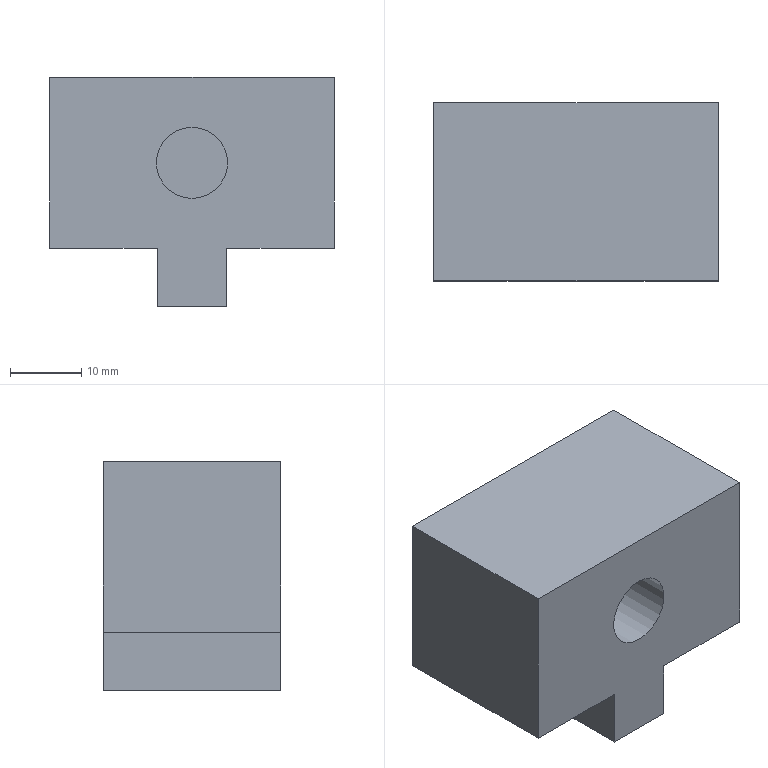Part | NX | features DATUM_CSYS 5, SIMPLE HOLE 4, SKETCH 4, HOLE PACKAGE 3, SYMBOLIC_THREAD 3, EXTRUDE 1 | 1 solid | 18 faces | box 40 x 25 x 32.2 mm | volume 24398 mm3 | plane 11 | cylinder 4 | cone 3 | commonest cylinder face diameters 4.2 x3 10 x1
STEP:
#1=CARTESIAN_POINT('',(-20.,0.,24.));
#2=VERTEX_POINT('',#1);
#3=CARTESIAN_POINT('',(-20.,0.,0.));
#4=VERTEX_POINT('',#3);
#5=CARTESIAN_POINT('',(-20.,0.,24.));
#6=DIRECTION('',(0.,0.,-1.));
#7=VECTOR('',#6,1000.);
#8=LINE('',#5,#7);
#9=EDGE_CURVE('',#2,#4,#8,.T.);
#10=ORIENTED_EDGE('',*,*,#9,.F.);
#11=CARTESIAN_POINT('',(-20.,25.,24.));
#12=VERTEX_POINT('',#11);
#13=CARTESIAN_POINT('',(-20.,25.,24.));
#14=DIRECTION('',(0.,-1.,0.));
#15=VECTOR('',#14,1000.);
#16=LINE('',#13,#15);
#17=EDGE_CURVE('',#12,#2,#16,.T.);
#18=ORIENTED_EDGE('',*,*,#17,.F.);
#19=CARTESIAN_POINT('',(-20.,25.,0.));
#20=VERTEX_POINT('',#19);
#21=CARTESIAN_POINT('',(-20.,25.,24.));
#22=DIRECTION('',(0.,0.,-1.));
#23=VECTOR('',#22,1000.);
#24=LINE('',#21,#23);
#25=EDGE_CURVE('',#12,#20,#24,.T.);
#26=ORIENTED_EDGE('',*,*,#25,.T.);
#27=CARTESIAN_POINT('',(-20.,25.,0.));
#28=DIRECTION('',(0.,-1.,0.));
#29=VECTOR('',#28,1000.);
#30=LINE('',#27,#29);
#31=EDGE_CURVE('',#20,#4,#30,.T.);
#32=ORIENTED_EDGE('',*,*,#31,.T.);
#33=EDGE_LOOP('',(#10,#18,#26,#32));
#34=FACE_BOUND('',#33,.T.);
#35=CARTESIAN_POINT('',(-20.,25.,24.));
#36=DIRECTION('',(-1.,0.,0.));
#37=DIRECTION('',(0.,0.,1.));
#38=AXIS2_PLACEMENT_3D('',#35,#36,#37);
#39=PLANE('',#38);
#40=ADVANCED_FACE('',(#34),#39,.T.);
#41=CARTESIAN_POINT('',(-4.9,0.,0.));
#42=VERTEX_POINT('',#41);
#43=CARTESIAN_POINT('',(-20.,0.,0.));
#44=DIRECTION('',(1.,0.,0.));
#45=VECTOR('',#44,1000.);
#46=LINE('',#43,#45);
#47=EDGE_CURVE('',#4,#42,#46,.T.);
#48=ORIENTED_EDGE('',*,*,#47,.F.);
#49=ORIENTED_EDGE('',*,*,#31,.F.);
#50=CARTESIAN_POINT('',(-4.9,25.,0.));
#51=VERTEX_POINT('',#50);
#52=CARTESIAN_POINT('',(-20.,25.,0.));
#53=DIRECTION('',(1.,0.,0.));
#54=VECTOR('',#53,1000.);
#55=LINE('',#52,#54);
#56=EDGE_CURVE('',#20,#51,#55,.T.);
#57=ORIENTED_EDGE('',*,*,#56,.T.);
#58=CARTESIAN_POINT('',(-4.9,25.,0.));
#59=DIRECTION('',(0.,-1.,0.));
#60=VECTOR('',#59,1000.);
#61=LINE('',#58,#60);
#62=EDGE_CURVE('',#51,#42,#61,.T.);
#63=ORIENTED_EDGE('',*,*,#62,.T.);
#64=EDGE_LOOP('',(#48,#49,#57,#63));
#65=FACE_BOUND('',#64,.T.);
#66=CARTESIAN_POINT('',(-20.,25.,0.));
#67=DIRECTION('',(0.,0.,-1.));
#68=DIRECTION('',(-1.,0.,0.));
#69=AXIS2_PLACEMENT_3D('',#66,#67,#68);
#70=PLANE('',#69);
#71=ADVANCED_FACE('',(#65),#70,.T.);
#72=CARTESIAN_POINT('',(-4.9,0.,-8.2));
#73=VERTEX_POINT('',#72);
#74=CARTESIAN_POINT('',(-4.9,0.,0.));
#75=DIRECTION('',(0.,0.,-1.));
#76=VECTOR('',#75,1000.);
#77=LINE('',#74,#76);
#78=EDGE_CURVE('',#42,#73,#77,.T.);
#79=ORIENTED_EDGE('',*,*,#78,.F.);
#80=ORIENTED_EDGE('',*,*,#62,.F.);
#81=CARTESIAN_POINT('',(-4.9,25.,-8.2));
#82=VERTEX_POINT('',#81);
#83=CARTESIAN_POINT('',(-4.9,25.,0.));
#84=DIRECTION('',(0.,0.,-1.));
#85=VECTOR('',#84,1000.);
#86=LINE('',#83,#85);
#87=EDGE_CURVE('',#51,#82,#86,.T.);
#88=ORIENTED_EDGE('',*,*,#87,.T.);
#89=CARTESIAN_POINT('',(-4.9,25.,-8.2));
#90=DIRECTION('',(0.,-1.,0.));
#91=VECTOR('',#90,1000.);
#92=LINE('',#89,#91);
#93=EDGE_CURVE('',#82,#73,#92,.T.);
#94=ORIENTED_EDGE('',*,*,#93,.T.);
#95=EDGE_LOOP('',(#79,#80,#88,#94));
#96=FACE_BOUND('',#95,.T.);
#97=CARTESIAN_POINT('',(-4.9,25.,0.));
#98=DIRECTION('',(-1.,0.,0.));
#99=DIRECTION('',(0.,0.,1.));
#100=AXIS2_PLACEMENT_3D('',#97,#98,#99);
#101=PLANE('',#100);
#102=ADVANCED_FACE('',(#96),#101,.T.);
#103=CARTESIAN_POINT('',(2.1,12.5,-8.2));
#104=VERTEX_POINT('',#103);
#105=CARTESIAN_POINT('',(0.,12.5,-8.2));
#106=DIRECTION('',(0.,0.,1.));
#107=DIRECTION('',(1.,0.,0.));
#108=AXIS2_PLACEMENT_3D('',#105,#106,#107);
#109=CIRCLE('',#108,2.1);
#110=EDGE_CURVE('',#104,#104,#109,.T.);
#111=ORIENTED_EDGE('',*,*,#110,.T.);
#112=EDGE_LOOP('',(#111));
#113=FACE_BOUND('',#112,.T.);
#114=CARTESIAN_POINT('',(4.9,0.,-8.2));
#115=VERTEX_POINT('',#114);
#116=CARTESIAN_POINT('',(-4.9,0.,-8.2));
#117=DIRECTION('',(1.,0.,0.));
#118=VECTOR('',#117,1000.);
#119=LINE('',#116,#118);
#120=EDGE_CURVE('',#73,#115,#119,.T.);
#121=ORIENTED_EDGE('',*,*,#120,.F.);
#122=ORIENTED_EDGE('',*,*,#93,.F.);
#123=CARTESIAN_POINT('',(4.9,25.,-8.2));
#124=VERTEX_POINT('',#123);
#125=CARTESIAN_POINT('',(-4.9,25.,-8.2));
#126=DIRECTION('',(1.,0.,0.));
#127=VECTOR('',#126,1000.);
#128=LINE('',#125,#127);
#129=EDGE_CURVE('',#82,#124,#128,.T.);
#130=ORIENTED_EDGE('',*,*,#129,.T.);
#131=CARTESIAN_POINT('',(4.9,25.,-8.2));
#132=DIRECTION('',(0.,-1.,0.));
#133=VECTOR('',#132,1000.);
#134=LINE('',#131,#133);
#135=EDGE_CURVE('',#124,#115,#134,.T.);
#136=ORIENTED_EDGE('',*,*,#135,.T.);
#137=EDGE_LOOP('',(#121,#122,#130,#136));
#138=FACE_BOUND('',#137,.T.);
#139=CARTESIAN_POINT('',(-4.9,25.,-8.2));
#140=DIRECTION('',(0.,0.,-1.));
#141=DIRECTION('',(-1.,0.,0.));
#142=AXIS2_PLACEMENT_3D('',#139,#140,#141);
#143=PLANE('',#142);
#144=ADVANCED_FACE('',(#113,#138),#143,.T.);
#145=CARTESIAN_POINT('',(4.9,0.,0.));
#146=VERTEX_POINT('',#145);
#147=CARTESIAN_POINT('',(4.9,0.,-8.2));
#148=DIRECTION('',(0.,0.,1.));
#149=VECTOR('',#148,1000.);
#150=LINE('',#147,#149);
#151=EDGE_CURVE('',#115,#146,#150,.T.);
#152=ORIENTED_EDGE('',*,*,#151,.F.);
#153=ORIENTED_EDGE('',*,*,#135,.F.);
#154=CARTESIAN_POINT('',(4.9,25.,0.));
#155=VERTEX_POINT('',#154);
#156=CARTESIAN_POINT('',(4.9,25.,-8.2));
#157=DIRECTION('',(0.,0.,1.));
#158=VECTOR('',#157,1000.);
#159=LINE('',#156,#158);
#160=EDGE_CURVE('',#124,#155,#159,.T.);
#161=ORIENTED_EDGE('',*,*,#160,.T.);
#162=CARTESIAN_POINT('',(4.9,25.,0.));
#163=DIRECTION('',(0.,-1.,0.));
#164=VECTOR('',#163,1000.);
#165=LINE('',#162,#164);
#166=EDGE_CURVE('',#155,#146,#165,.T.);
#167=ORIENTED_EDGE('',*,*,#166,.T.);
#168=EDGE_LOOP('',(#152,#153,#161,#167));
#169=FACE_BOUND('',#168,.T.);
#170=CARTESIAN_POINT('',(4.9,25.,-8.2));
#171=DIRECTION('',(1.,0.,0.));
#172=DIRECTION('',(0.,0.,-1.));
#173=AXIS2_PLACEMENT_3D('',#170,#171,#172);
#174=PLANE('',#173);
#175=ADVANCED_FACE('',(#169),#174,.T.);
#176=CARTESIAN_POINT('',(20.,0.,0.));
#177=VERTEX_POINT('',#176);
#178=CARTESIAN_POINT('',(4.9,0.,0.));
#179=DIRECTION('',(1.,0.,0.));
#180=VECTOR('',#179,1000.);
#181=LINE('',#178,#180);
#182=EDGE_CURVE('',#146,#177,#181,.T.);
#183=ORIENTED_EDGE('',*,*,#182,.F.);
#184=ORIENTED_EDGE('',*,*,#166,.F.);
#185=CARTESIAN_POINT('',(20.,25.,0.));
#186=VERTEX_POINT('',#185);
#187=CARTESIAN_POINT('',(4.9,25.,0.));
#188=DIRECTION('',(1.,0.,0.));
#189=VECTOR('',#188,1000.);
#190=LINE('',#187,#189);
#191=EDGE_CURVE('',#155,#186,#190,.T.);
#192=ORIENTED_EDGE('',*,*,#191,.T.);
#193=CARTESIAN_POINT('',(20.,25.,0.));
#194=DIRECTION('',(0.,-1.,0.));
#195=VECTOR('',#194,1000.);
#196=LINE('',#193,#195);
#197=EDGE_CURVE('',#186,#177,#196,.T.);
#198=ORIENTED_EDGE('',*,*,#197,.T.);
#199=EDGE_LOOP('',(#183,#184,#192,#198));
#200=FACE_BOUND('',#199,.T.);
#201=CARTESIAN_POINT('',(4.9,25.,0.));
#202=DIRECTION('',(0.,0.,-1.));
#203=DIRECTION('',(-1.,0.,0.));
#204=AXIS2_PLACEMENT_3D('',#201,#202,#203);
#205=PLANE('',#204);
#206=ADVANCED_FACE('',(#200),#205,.T.);
#207=CARTESIAN_POINT('',(20.,0.,24.));
#208=VERTEX_POINT('',#207);
#209=CARTESIAN_POINT('',(20.,0.,0.));
#210=DIRECTION('',(0.,0.,1.));
#211=VECTOR('',#210,1000.);
#212=LINE('',#209,#211);
#213=EDGE_CURVE('',#177,#208,#212,.T.);
#214=ORIENTED_EDGE('',*,*,#213,.F.);
#215=ORIENTED_EDGE('',*,*,#197,.F.);
#216=CARTESIAN_POINT('',(20.,25.,24.));
#217=VERTEX_POINT('',#216);
#218=CARTESIAN_POINT('',(20.,25.,0.));
#219=DIRECTION('',(0.,0.,1.));
#220=VECTOR('',#219,1000.);
#221=LINE('',#218,#220);
#222=EDGE_CURVE('',#186,#217,#221,.T.);
#223=ORIENTED_EDGE('',*,*,#222,.T.);
#224=CARTESIAN_POINT('',(20.,25.,24.));
#225=DIRECTION('',(0.,-1.,0.));
#226=VECTOR('',#225,1000.);
#227=LINE('',#224,#226);
#228=EDGE_CURVE('',#217,#208,#227,.T.);
#229=ORIENTED_EDGE('',*,*,#228,.T.);
#230=EDGE_LOOP('',(#214,#215,#223,#229));
#231=FACE_BOUND('',#230,.T.);
#232=CARTESIAN_POINT('',(20.,25.,0.));
#233=DIRECTION('',(1.,0.,0.));
#234=DIRECTION('',(0.,0.,-1.));
#235=AXIS2_PLACEMENT_3D('',#232,#233,#234);
#236=PLANE('',#235);
#237=ADVANCED_FACE('',(#231),#236,.T.);
#238=CARTESIAN_POINT('',(20.,0.,24.));
#239=DIRECTION('',(-1.,0.,0.));
#240=VECTOR('',#239,1000.);
#241=LINE('',#238,#240);
#242=EDGE_CURVE('',#208,#2,#241,.T.);
#243=ORIENTED_EDGE('',*,*,#242,.F.);
#244=ORIENTED_EDGE('',*,*,#228,.F.);
#245=CARTESIAN_POINT('',(20.,25.,24.));
#246=DIRECTION('',(-1.,0.,0.));
#247=VECTOR('',#246,1000.);
#248=LINE('',#245,#247);
#249=EDGE_CURVE('',#217,#12,#248,.T.);
#250=ORIENTED_EDGE('',*,*,#249,.T.);
#251=ORIENTED_EDGE('',*,*,#17,.T.);
#252=EDGE_LOOP('',(#243,#244,#250,#251));
#253=FACE_BOUND('',#252,.T.);
#254=CARTESIAN_POINT('',(20.,25.,24.));
#255=DIRECTION('',(0.,0.,1.));
#256=DIRECTION('',(1.,0.,0.));
#257=AXIS2_PLACEMENT_3D('',#254,#255,#256);
#258=PLANE('',#257);
#259=ADVANCED_FACE('',(#253),#258,.T.);
#260=CARTESIAN_POINT('',(12.,25.,9.9));
#261=VERTEX_POINT('',#260);
#262=CARTESIAN_POINT('',(12.,25.,12.));
#263=DIRECTION('',(0.,-1.,0.));
#264=DIRECTION('',(0.,0.,-1.));
#265=AXIS2_PLACEMENT_3D('',#262,#263,#264);
#266=CIRCLE('',#265,2.1);
#267=EDGE_CURVE('',#261,#261,#266,.T.);
#268=ORIENTED_EDGE('',*,*,#267,.T.);
#269=EDGE_LOOP('',(#268));
#270=FACE_BOUND('',#269,.T.);
#271=CARTESIAN_POINT('',(-12.,25.,9.9));
#272=VERTEX_POINT('',#271);
#273=CARTESIAN_POINT('',(-12.,25.,12.));
#274=DIRECTION('',(0.,-1.,0.));
#275=DIRECTION('',(0.,0.,-1.));
#276=AXIS2_PLACEMENT_3D('',#273,#274,#275);
#277=CIRCLE('',#276,2.1);
#278=EDGE_CURVE('',#272,#272,#277,.T.);
#279=ORIENTED_EDGE('',*,*,#278,.T.);
#280=EDGE_LOOP('',(#279));
#281=FACE_BOUND('',#280,.T.);
#282=ORIENTED_EDGE('',*,*,#25,.F.);
#283=ORIENTED_EDGE('',*,*,#249,.F.);
#284=ORIENTED_EDGE('',*,*,#222,.F.);
#285=ORIENTED_EDGE('',*,*,#191,.F.);
#286=ORIENTED_EDGE('',*,*,#160,.F.);
#287=ORIENTED_EDGE('',*,*,#129,.F.);
#288=ORIENTED_EDGE('',*,*,#87,.F.);
#289=ORIENTED_EDGE('',*,*,#56,.F.);
#290=EDGE_LOOP('',(#282,#283,#284,#285,#286,#287,#288,#289));
#291=FACE_BOUND('',#290,.T.);
#292=CARTESIAN_POINT('',(0.,25.,0.));
#293=DIRECTION('',(0.,-1.,0.));
#294=DIRECTION('',(0.,0.,-1.));
#295=AXIS2_PLACEMENT_3D('',#292,#293,#294);
#296=PLANE('',#295);
#297=ADVANCED_FACE('',(#270,#281,#291),#296,.F.);
#298=CARTESIAN_POINT('',(0.,0.,17.));
#299=VERTEX_POINT('',#298);
#300=CARTESIAN_POINT('',(0.,0.,12.));
#301=DIRECTION('',(0.,1.,0.));
#302=DIRECTION('',(0.,0.,1.));
#303=AXIS2_PLACEMENT_3D('',#300,#301,#302);
#304=CIRCLE('',#303,5.);
#305=EDGE_CURVE('',#299,#299,#304,.T.);
#306=ORIENTED_EDGE('',*,*,#305,.T.);
#307=EDGE_LOOP('',(#306));
#308=FACE_BOUND('',#307,.T.);
#309=ORIENTED_EDGE('',*,*,#9,.T.);
#310=ORIENTED_EDGE('',*,*,#47,.T.);
#311=ORIENTED_EDGE('',*,*,#78,.T.);
#312=ORIENTED_EDGE('',*,*,#120,.T.);
#313=ORIENTED_EDGE('',*,*,#151,.T.);
#314=ORIENTED_EDGE('',*,*,#182,.T.);
#315=ORIENTED_EDGE('',*,*,#213,.T.);
#316=ORIENTED_EDGE('',*,*,#242,.T.);
#317=EDGE_LOOP('',(#309,#310,#311,#312,#313,#314,#315,#316));
#318=FACE_BOUND('',#317,.T.);
#319=CARTESIAN_POINT('',(0.,0.,0.));
#320=DIRECTION('',(0.,-1.,0.));
#321=DIRECTION('',(0.,0.,-1.));
#322=AXIS2_PLACEMENT_3D('',#319,#320,#321);
#323=PLANE('',#322);
#324=ADVANCED_FACE('',(#308,#318),#323,.T.);
#325=CARTESIAN_POINT('',(0.,15.,17.));
#326=VERTEX_POINT('',#325);
#327=CARTESIAN_POINT('',(0.,15.,12.));
#328=DIRECTION('',(0.,1.,0.));
#329=DIRECTION('',(0.,0.,1.));
#330=AXIS2_PLACEMENT_3D('',#327,#328,#329);
#331=CIRCLE('',#330,5.);
#332=EDGE_CURVE('',#326,#326,#331,.F.);
#333=ORIENTED_EDGE('',*,*,#332,.T.);
#334=EDGE_LOOP('',(#333));
#335=FACE_BOUND('',#334,.T.);
#336=CARTESIAN_POINT('',(0.,15.,12.));
#337=DIRECTION('',(0.,1.,0.));
#338=DIRECTION('',(0.,0.,1.));
#339=AXIS2_PLACEMENT_3D('',#336,#337,#338);
#340=PLANE('',#339);
#341=ADVANCED_FACE('',(#335),#340,.F.);
#342=ORIENTED_EDGE('',*,*,#332,.F.);
#343=EDGE_LOOP('',(#342));
#344=FACE_BOUND('',#343,.T.);
#345=ORIENTED_EDGE('',*,*,#305,.F.);
#346=EDGE_LOOP('',(#345));
#347=FACE_BOUND('',#346,.T.);
#348=CARTESIAN_POINT('',(0.,0.,12.));
#349=DIRECTION('',(0.,1.,0.));
#350=DIRECTION('',(0.,0.,1.));
#351=AXIS2_PLACEMENT_3D('',#348,#349,#350);
#352=CYLINDRICAL_SURFACE('',#351,5.);
#353=ADVANCED_FACE('',(#344,#347),#352,.F.);
#354=CARTESIAN_POINT('',(-12.,15.,9.9));
#355=VERTEX_POINT('',#354);
#356=CARTESIAN_POINT('',(-12.,15.,12.));
#357=DIRECTION('',(0.,-1.,0.));
#358=DIRECTION('',(0.,0.,-1.));
#359=AXIS2_PLACEMENT_3D('',#356,#357,#358);
#360=CIRCLE('',#359,2.1);
#361=EDGE_CURVE('',#355,#355,#360,.F.);
#362=ORIENTED_EDGE('',*,*,#361,.T.);
#363=EDGE_LOOP('',(#362));
#364=FACE_BOUND('',#363,.T.);
#365=CARTESIAN_POINT('',(-12.,13.738,12.));
#366=VERTEX_POINT('',#365);
#367=VERTEX_LOOP('',#366);
#368=FACE_BOUND('',#367,.T.);
#369=CARTESIAN_POINT('',(-12.,15.,12.));
#370=DIRECTION('',(0.,1.,0.));
#371=DIRECTION('',(0.,0.,1.));
#372=AXIS2_PLACEMENT_3D('',#369,#370,#371);
#373=CONICAL_SURFACE('',#372,2.1,1.03);
#374=ADVANCED_FACE('',(#364,#368),#373,.F.);
#375=ORIENTED_EDGE('',*,*,#361,.F.);
#376=EDGE_LOOP('',(#375));
#377=FACE_BOUND('',#376,.T.);
#378=ORIENTED_EDGE('',*,*,#278,.F.);
#379=EDGE_LOOP('',(#378));
#380=FACE_BOUND('',#379,.T.);
#381=CARTESIAN_POINT('',(-12.,25.,12.));
#382=DIRECTION('',(0.,-1.,0.));
#383=DIRECTION('',(0.,0.,-1.));
#384=AXIS2_PLACEMENT_3D('',#381,#382,#383);
#385=CYLINDRICAL_SURFACE('',#384,2.1);
#386=ADVANCED_FACE('',(#377,#380),#385,.F.);
#387=CARTESIAN_POINT('',(12.,15.,9.9));
#388=VERTEX_POINT('',#387);
#389=CARTESIAN_POINT('',(12.,15.,12.));
#390=DIRECTION('',(0.,-1.,0.));
#391=DIRECTION('',(0.,0.,-1.));
#392=AXIS2_PLACEMENT_3D('',#389,#390,#391);
#393=CIRCLE('',#392,2.1);
#394=EDGE_CURVE('',#388,#388,#393,.F.);
#395=ORIENTED_EDGE('',*,*,#394,.T.);
#396=EDGE_LOOP('',(#395));
#397=FACE_BOUND('',#396,.T.);
#398=CARTESIAN_POINT('',(12.,13.738,12.));
#399=VERTEX_POINT('',#398);
#400=VERTEX_LOOP('',#399);
#401=FACE_BOUND('',#400,.T.);
#402=CARTESIAN_POINT('',(12.,15.,12.));
#403=DIRECTION('',(0.,1.,0.));
#404=DIRECTION('',(0.,0.,1.));
#405=AXIS2_PLACEMENT_3D('',#402,#403,#404);
#406=CONICAL_SURFACE('',#405,2.1,1.03);
#407=ADVANCED_FACE('',(#397,#401),#406,.F.);
#408=ORIENTED_EDGE('',*,*,#394,.F.);
#409=EDGE_LOOP('',(#408));
#410=FACE_BOUND('',#409,.T.);
#411=ORIENTED_EDGE('',*,*,#267,.F.);
#412=EDGE_LOOP('',(#411));
#413=FACE_BOUND('',#412,.T.);
#414=CARTESIAN_POINT('',(12.,25.,12.));
#415=DIRECTION('',(0.,-1.,0.));
#416=DIRECTION('',(0.,0.,-1.));
#417=AXIS2_PLACEMENT_3D('',#414,#415,#416);
#418=CYLINDRICAL_SURFACE('',#417,2.1);
#419=ADVANCED_FACE('',(#410,#413),#418,.F.);
#420=CARTESIAN_POINT('',(2.1,12.5,1.8));
#421=VERTEX_POINT('',#420);
#422=CARTESIAN_POINT('',(0.,12.5,1.8));
#423=DIRECTION('',(0.,0.,1.));
#424=DIRECTION('',(1.,0.,0.));
#425=AXIS2_PLACEMENT_3D('',#422,#423,#424);
#426=CIRCLE('',#425,2.1);
#427=EDGE_CURVE('',#421,#421,#426,.F.);
#428=ORIENTED_EDGE('',*,*,#427,.T.);
#429=EDGE_LOOP('',(#428));
#430=FACE_BOUND('',#429,.T.);
#431=CARTESIAN_POINT('',(0.,12.5,3.062));
#432=VERTEX_POINT('',#431);
#433=VERTEX_LOOP('',#432);
#434=FACE_BOUND('',#433,.T.);
#435=CARTESIAN_POINT('',(0.,12.5,1.8));
#436=DIRECTION('',(0.,0.,-1.));
#437=DIRECTION('',(-1.,0.,0.));
#438=AXIS2_PLACEMENT_3D('',#435,#436,#437);
#439=CONICAL_SURFACE('',#438,2.1,1.03);
#440=ADVANCED_FACE('',(#430,#434),#439,.F.);
#441=ORIENTED_EDGE('',*,*,#427,.F.);
#442=EDGE_LOOP('',(#441));
#443=FACE_BOUND('',#442,.T.);
#444=ORIENTED_EDGE('',*,*,#110,.F.);
#445=EDGE_LOOP('',(#444));
#446=FACE_BOUND('',#445,.T.);
#447=CARTESIAN_POINT('',(0.,12.5,-8.2));
#448=DIRECTION('',(0.,0.,1.));
#449=DIRECTION('',(1.,0.,0.));
#450=AXIS2_PLACEMENT_3D('',#447,#448,#449);
#451=CYLINDRICAL_SURFACE('',#450,2.1);
#452=ADVANCED_FACE('',(#443,#446),#451,.F.);
#453=CLOSED_SHELL('',(#40,#71,#102,#144,#175,#206,#237,#259,#297,#324,#341,#353,#374,#386,#407,#419,#440,#452));
#454=MANIFOLD_SOLID_BREP('',#453);
#455=(LENGTH_UNIT()NAMED_UNIT(*)SI_UNIT(.MILLI.,.METRE.));
#456=UNCERTAINTY_MEASURE_WITH_UNIT(LENGTH_MEASURE(0.00001),#455,'','');
#457=(NAMED_UNIT(*)PLANE_ANGLE_UNIT()SI_UNIT($,.RADIAN.));
#458=(NAMED_UNIT(*)SI_UNIT($,.STERADIAN.)SOLID_ANGLE_UNIT());
#459=(GEOMETRIC_REPRESENTATION_CONTEXT(3)GLOBAL_UNCERTAINTY_ASSIGNED_CONTEXT((#456))GLOBAL_UNIT_ASSIGNED_CONTEXT((#455,#457,#458))REPRESENTATION_CONTEXT('',''));
#460=ADVANCED_BREP_SHAPE_REPRESENTATION('',(#454),#459);